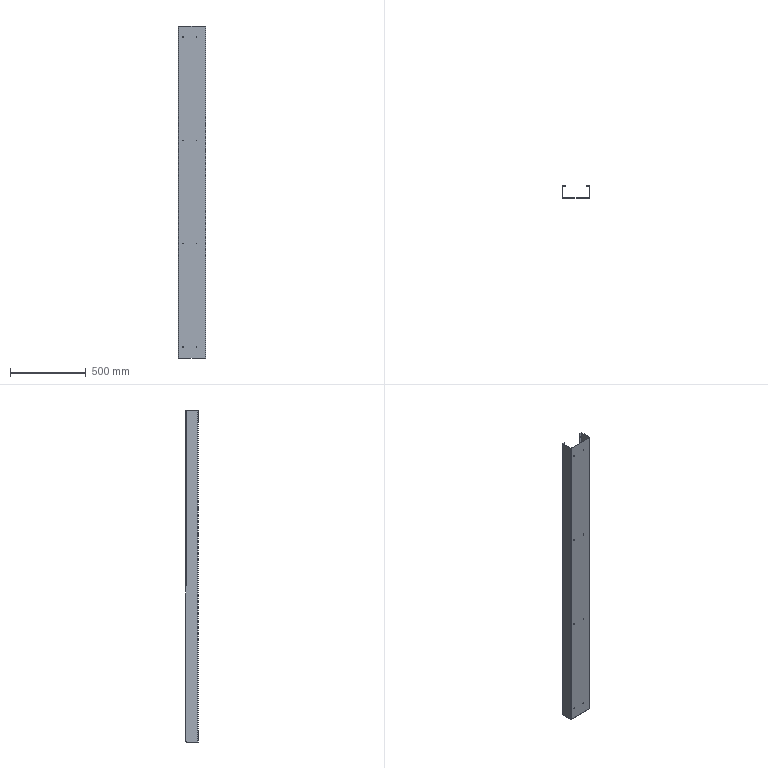Part | SolidWorks | features ICE 2, LPattern 2, SMMiteredFlange 2, Chamfer 1, Fillet 1, FlatPattern 1, SMBaseFlange 1, SheetMetal 1 | 1 solid | 80 faces | box 180 x 80 x 2190 mm | volume 1160945 mm3 | plane 38 | cylinder 26 | cone 16 | commonest cylinder face diameters 6.4 x12 4 x6 3 x4 6 x4